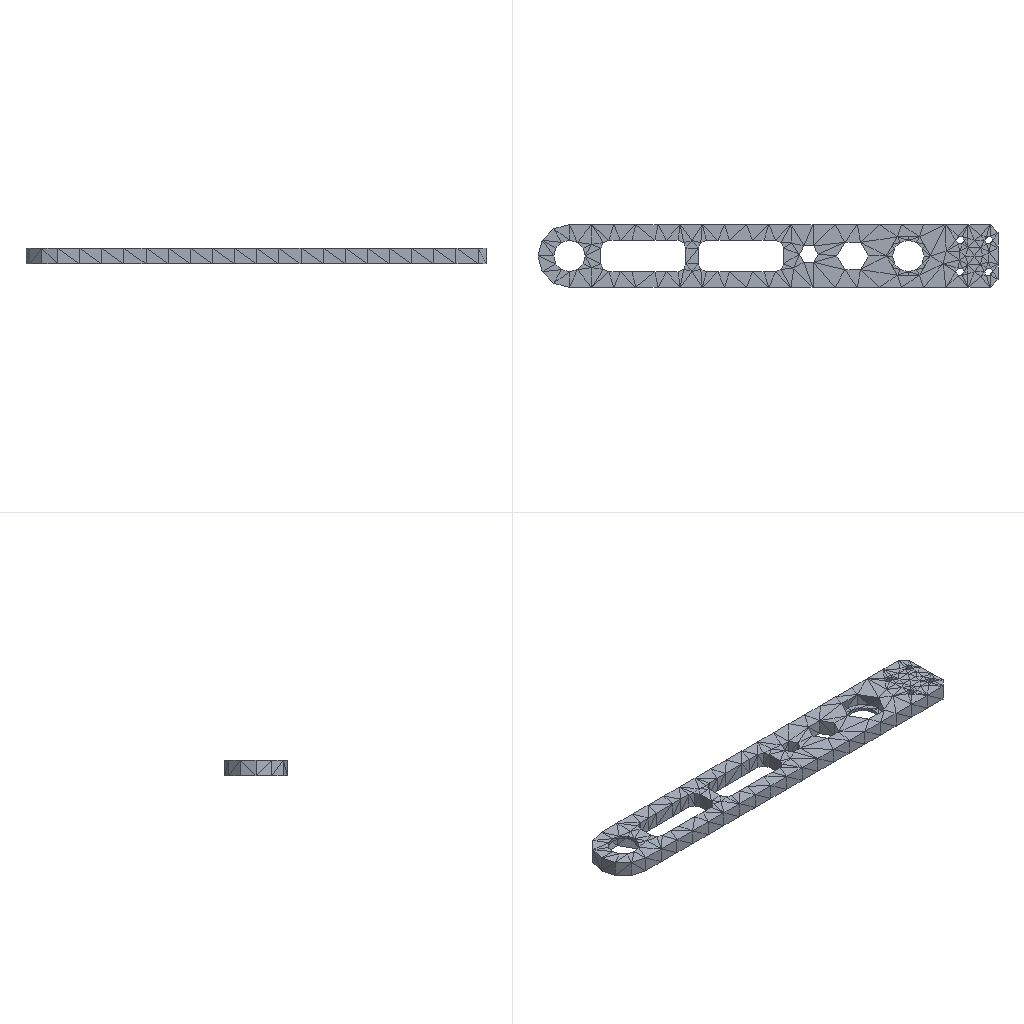Simulation study | ansys workbench
Ansys APDL input file, long lists of numbers shortened:
/batch
/config,noeldb,1     ! force off writing results to database
*get,_wallstrt,active,,time,wall
! ANSYS input file written by Workbench version 2022 R1
! File used for geometry attach: F:\ansys（分析文件汇总)\轴机械结构有限元分析\交付(1)\交付\凸轮从动件.STEP
/title,wbnew--____ (F5)
! ****** Begin Custom Load Command Snippet ******
/COM, ACT Extensions:
/COM,     LSDYNA, 2021.1
/COM,
! ****** End   Custom Load Command Snippet ******
*DIM,_wb_ProjectScratch_dir,string,248
_wb_ProjectScratch_dir(1) = 'C:\Users\Administrator\AppData\Local\Temp\WB_Administrator_11372_2\_ProjectScratch\ScrC51E\'
*DIM,_wb_SolverFiles_dir,string,248
_wb_SolverFiles_dir(1) = 'C:\Users\Administrator\AppData\Local\Temp\WB_Administrator_11372_2\wbnew_files\dp0\SYS-2\MECH\'
*DIM,_wb_userfiles_dir,string,248
_wb_userfiles_dir(1) = 'C:\Users\Administrator\AppData\Local\Temp\WB_Administrator_11372_2\wbnew_files\user_files\'
/com,--- Data in consistent NMM units. See Solving Units in the help system for more information.
/units,MPA
/nopr
/wb,file,start              !  signify a WB generated input file
/prep7
! Turn off shape checking because checks already performed inside WB mesher.
! See help system for more information.
SHPP,OFF,,NOWARN
/nolist
etcon,set             ! allow ANSYS to choose best KEYOP's for 180x elements, resets any applicable keyopt to MAPDL defaults
/com,*********** Nodes for the whole assembly ***********
nblock,3,,2642
(1i9,3e20.9e3)
        1     2.000000000E+01    -5.000000000E+00    -5.000000000E+00
! (2401 more lines like these left out)
-1
/wb,elem,start            !  set before creation of elements
/com,*********** Elements for Body 1 "_____-FreeParts|NONE" ***********
et,1,187
eblock,19,solid,,1086
(19i9)
        1        1        1        1        0        0        0        0       10        0        1      238      442      310      308     1783     2037     1782     1781
! (2171 more lines like these left out)
-1
/wb,elem,end               !  done creating elements
/com,*********** Send User Defined Coordinate System(s) ***********
csys,0
toffst,273.15,  ! Temperature offset from absolute zero
/com,*********** Set Reference Temperature ***********
tref,22.
/wb,mat,start              !  starting to send materials
/com,*********** Send Materials ***********
Temperature = 'TEMP' ! Temperature
MP,DENS,1,7.85e-09,	! tonne mm^-3
MP,ALPX,1,1.2e-05,	! C^-1
MP,C,1,434000000,	! mm^2 s^-2 C^-1
MP,KXX,1,60.5,	! tonne mm s^-3 C^-1
MP,RSVX,1,0.00017,	! ohm mm
MP,EX,1,200000,	! tonne s^-2 mm^-1
MP,NUXY,1,0.3,
MP,MURX,1,10000,
/wb,mat,end                !  done sending materials
!************************* Model Summary ********************
!_____-FreeParts|NONE,	结构钢,	matid,	1
!************************* End Model Summary ********************
! get the diagonal of the bounding box. Needed later for other things
*get,_xmin,node,,mnloc,x
*get,_ymin,node,,mnloc,y
*get,_zmin,node,,mnloc,z
*get,_xmax,node,,mxloc,x
*get,_ymax,node,,mxloc,y
*get,_zmax,node,,mxloc,z
_ASMDIAG=(_xmax-_xmin)*(_xmax-_xmin)+(_ymax-_ymin)*(_ymax-_ymin)+(_zmax-_zmin)*(_zmax-_zmin)
_ASMDIAG=SQRT(_ASMDIAG)
/wb,contact,start          !  starting to send contact
/wb,contact,end            !  done creating contacts
/golist
/wb,load,start             !  starting to send loads
/com,*********** Fixed Supports ***********
CMBLOCK,_FIXEDSU,NODE,      280
(8i10)
        65        66        67        68        69        70        71        72
! (34 more lines like these left out)
cmsel,s,_FIXEDSU
d,all,all
nsel,all
/com,*********** Define Force Using Surface Effect Elements ***********
local,12,0,0.,0.,0.,0.,0.,0.
csys,0
et,2,154
eblock,10,,,211
(15i9)
     1933        2        2        2       12       16      239       18       18      536      547       18      535
! (210 more lines like these left out)
-1
esel,s,type,,2
keyop,2,2,1                ! Apply load in local coordinate system
keyop,2,7,1                ! Use original area so load is constant in large deformation
esel,all
/gst,on,on
fini
*get,_numnode,node,0,count
*get,_numelem,elem,0,count
*get, _MAXELEMNUM, elem, 0, NUM, MAX
*get, _MAXNODENUM, node, 0, NUM, MAX
*get, _MAXELEMTYPE, etyp, 0, NUM, MAX
*get, _MAXREALCONST, real, 0, NUM, MAX
/go
/wb,load,end               !  done creating loads
/com,--- Number of total nodes = %_numnode%
/com,--- Number of contact elements = 211
/com,--- Number of spring elements = 0
/com,--- Number of bearing elements = 0
/com,--- Number of solid elements = 1086
/com,--- Number of condensed parts = 0
/com,--- Number of total elements = %_numelem%
*get,_wallbsol,active,,time,wall
/com,****************************************************************************
/com,*************************    SOLUTION       ********************************
/com,****************************************************************************
/solu
antype,0                   ! static analysis
_thickRatio=  0     ! Ratio of thick parts in the model
eqsl,sparse,,,,,1
cntr,print,1               ! print out contact info and also make no initial contact an error
dmpoption,emat,no             ! Don't combine emat file for DANSYS
dmpoption,esav,no             ! Don't combine esav file for DANSYS
nldiag,cont,iter           ! print out contact info each equilibrium iteration
rescontrol,,none                 ! Do not keep any restart files
/com,****************************************************
/com,******************* SOLVE FOR LS 1 OF 1 ****************
esel,s,type,,2
nsle
sfe,all,1,pres,1,0.
sfe,all,2,pres,1,0.
sfe,all,3,pres,1,-0.126
nsel,all
esel,all
/nopr
/gopr
nsub,1,1,1
time,1.
outres,erase
outres,all,none
outres,nsol,all,
outres,rsol,all
outres,eangl,all
outres,etmp,all
outres,veng,all
outres,strs,all,
outres,epel,all,
outres,eppl,all,
outres,cont,all,
! *********** WB SOLVE COMMAND ***********
! check interactive state
*get,ANSINTER_,active,,int
*if,ANSINTER_,ne,0,then
/eof
*endif
solve
/com *************** Write FE CONNECTORS *********
CEWRITE,file,ce,,INTE
/com,****************************************************
/com,*************** FINISHED SOLVE FOR LS 1 *************
*get,_wallasol,active,,time,wall
/nopr
*get,_numnode,node,0,count
*get,_numelem,elem,0,count
*get, _MAXELEMNUM, elem, 0, NUM, MAX
*get, _MAXNODENUM, node, 0, NUM, MAX,,,INTERNAL
*get, _MAXELEMTYPE, etyp, 0, NUM, MAX
*get, _MAXREALCONST, real, 0, NUM, MAX
/gopr
/post1
xmlo,ENCODING,ISO-8859-1
xmlo,parm
/xml,parm,xml
fini
/gopr
*get,_walldone,active,,time,wall
_preptime=(_wallbsol-_wallstrt)*3600
_solvtime=(_wallasol-_wallbsol)*3600
_posttime=(_walldone-_wallasol)*3600
_totaltim=(_walldone-_wallstrt)*3600
*get,_dlbratio,active,0,solu,dlbr
*get,_combtime,active,0,solu,comb
*get,_ssmode,active,0,solu,ssmm
*get,_ndofs,active,0,solu,ndof
*get,_sol_end_time,active,0,set,time
*if,_sol_end_time,eq,1.,then
/fclean				!clean distributed files
*endif
/com,--- Total number of nodes = %_numnode%
/com,--- Total number of elements = %_numelem%
/com,--- Element load balance ratio = %_dlbratio%
/com,--- Time to combine distributed files = %_combtime%
/com,--- Sparse memory mode = %_ssmode%
/com,--- Number of DOF = %_ndofs%
/wb,file,end               ! done with WB generated input